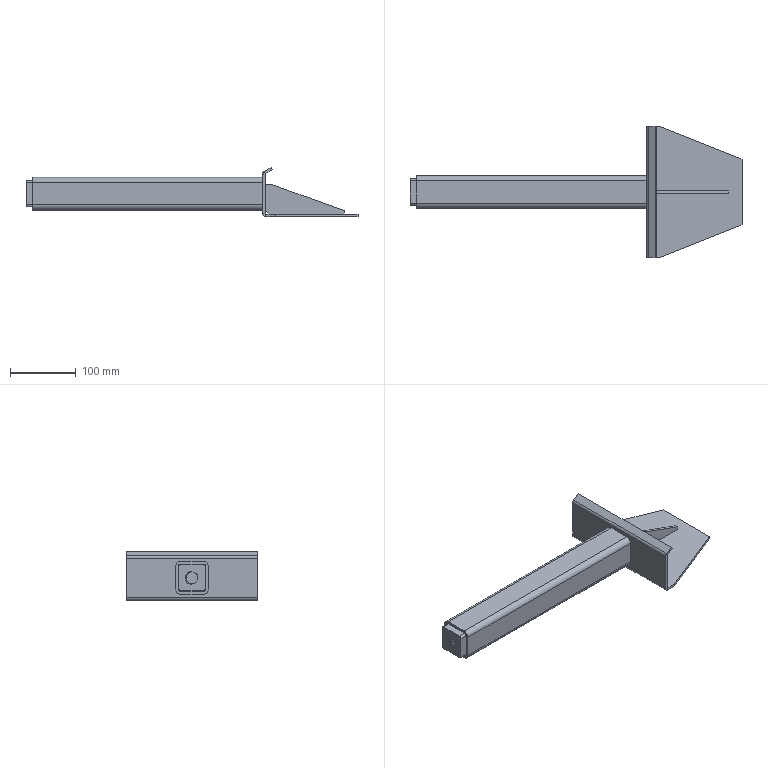Part | SolidWorks | features ICE 3, EdgeFlange 2, FlatPattern 1, Gusset 1, SMBaseFlange 1, SheetMetal 1, SweepThread 1, WeldMemberFeat 1, WeldmentFeature 1 | 4 solids | 85 faces | box 505 x 200 x 74.971 mm | volume 438985 mm3 | plane 45 | cylinder 37 | spline 3 | commonest cylinder face diameters 18 x21 6 x4 8 x4 16 x4 1.473 x2 9.473 x2